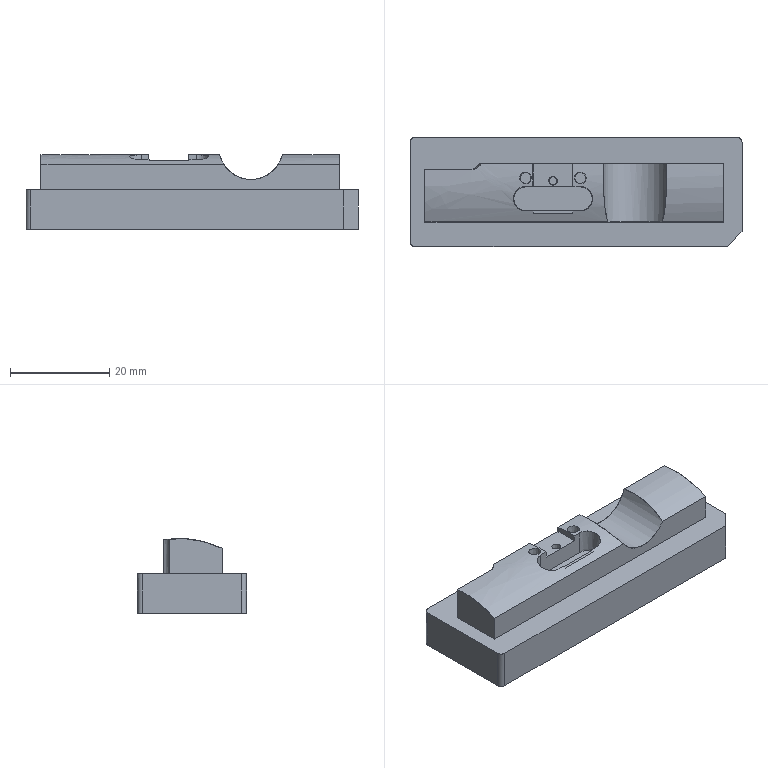NC program | PowerMill | posted with a generic post | part box 67 x 22 x 15.086 mm
Lines 3683 to 4683 of 148586:
N3780 M6
N3781 S18000 M03
N3782 G00 G90 X0.0 Y0.0
N3783 G43 Z9.7955 H15
N3784
N3785 G05 P10000 R4
N3786 X-0.8696 Y7.2678
N3787 Z0.7184
N3788 G01 Z-0.4816 F3000.0
N3789 X-0.8635 Y7.0754 F5000.0
N3790 X-0.8443 Y6.4662
N3791 X-0.4221 Y6.4795
N3792 X5.4877 Y6.4791
N3793 X5.9099 Y6.4424
N3794 X6.332 Y6.2619
N3795 X6.699 Y5.9099
N3796 X6.7541 Y5.8301
N3797 X6.9017 Y5.4877
N3798 X6.9594 Y5.0656
N3799 X6.9493 Y0.0
N3800 X6.8266 Y-0.4221
N3801 X6.7541 Y-0.5606
N3802 X6.5112 Y-0.8443
N3803 X6.332 Y-0.9949
N3804 X5.9099 Y-1.1709
N3805 X5.4877 Y-1.2145
N3806 X2.9549 Y-1.2306
N3807 X2.5328 Y-1.2027
N3808 X2.1107 Y-1.0409
N3809 X1.845 Y-0.8443
N3810 X1.5425 Y-0.5315
N3811 X1.2664 Y-0.3711
N3812 X0.8443 Y-0.2921
N3813 X0.8317 Y-0.2919
N3814 X0.8315
N3815 X-0.8443 Y-0.2674
N3816 X-1.2664 Y-0.1398
N3817 X-1.4842 Y0.0
N3818 X-1.6885 Y0.1971
N3819 X-1.8424 Y0.4221
N3820 X-1.9943 Y0.8443
N3821 X-2.0149 Y1.2664
N3822 X-2.0147 Y2.9871
N3823 X-4.0313 Y2.9866
N3824 G02 X-4.4729 Y2.5458 I-0.4407 J-0.0001
N3825 G01 X-4.8546 Y2.5466
N3826 G02 X-5.2944 Y2.988 I0.0009 J0.4407
N3827 G01 X-5.2942 Y3.1438
N3828 G02 X-4.8538 Y3.5838 I0.4407 J-0.0007
N3829 G01 X-4.4724 Y3.5841
N3830 G02 X-4.0314 Y3.1435 I0.0003 J-0.4407
N3831 G01 X-4.0313 Y2.9866
N3832 X-2.0147 Y2.9871
N3833 X-2.0145 Y5.0656
N3834 X-1.9606 Y5.4877
N3835 X-1.6885 Y5.9979
N3836 X-1.259 Y6.332
N3837 X-0.8443 Y6.4662
N3838 X-0.8635 Y7.0754
N3839 G00 Z3.8484
N3840 G01 X-13.9303 Y7.2926 F10000.0
N3841 G00 Z0.7184
N3842 G01 Z-0.4816 F3000.0
N3843 Y7.1001 F5000.0
N3844 X-13.9304 Y6.48
N3845 X-8.8648 Y6.4793
N3846 X-8.4427 Y6.46
N3847 X-8.0644 Y6.332
N3848 X-7.5984 Y5.9509
N3849 X-7.3648 Y5.4877
N3850 X-7.3108 Y5.0656
N3851 X-7.3106 Y1.2664
N3852 X-7.3319 Y0.8443
N3853 X-7.4812 Y0.4221
N3854 X-7.5984 Y0.2412
N3855 X-7.8433 Y0.0
N3856 X-8.0205 Y-0.1176
N3857 X-8.4427 Y-0.2668
N3858 X-10.1312 Y-0.2895
N3859 X-10.1441 Y-0.2919
N3860 X-10.5533 Y-0.3695
N3861 X-10.8312 Y-0.5295
N3862 X-11.1356 Y-0.8443
N3863 X-11.3976 Y-1.04
N3864 X-11.8197 Y-1.2005
N3865 X-12.2419 Y-1.23
N3866 X-18.5739 Y-1.1939
N3867 X-22.3731 Y-1.132
N3868 X-29.7609 Y-1.1249
N3869 X-30.3936 Y-1.2076
N3870 X-30.8157 Y-1.1609
N3871 X-31.2379 Y-0.9742
N3872 X-31.4044 Y-0.8443
N3873 X-31.66 Y-0.5304
N3874 X-31.7151 Y-0.4221
N3875 X-31.8364 Y0.0
N3876 X-31.8467 Y0.4221
N3877 Y4.2213
N3878 X-31.8399 Y4.6435
N3879 X-31.7279 Y5.0656
N3880 X-31.66 Y5.198
N3881 X-31.4339 Y5.4877
N3882 X-31.2379 Y5.6466
N3883 X-30.8157 Y5.8349
N3884 X-30.3936 Y5.8775
N3885 X-21.1067
N3886 X-21.0966 Y5.8789
N3887 X-20.8747 Y5.9099
N3888 X-20.6845 Y5.9891
N3889 X-20.2624 Y6.3017
N3890 X-19.8403 Y6.4525
N3891 X-18.996 Y6.4808
N3892 X-13.9304 Y6.48
N3893 X-13.9303 Y7.1001
N3894 G00 Z3.7118
N3895 G01 X-1.7244 Y-0.8629 F10000.0
N3896 G00 Z0.5818
N3897 G01 Z-0.6182 F3000.0
N3898 X-1.6213 Y-0.7004 F5000.0
N3899 X-1.2664 Y-0.1409
N3900 X-1.4885 Y0.0
N3901 X-1.6885 Y0.1953
N3902 X-1.8436 Y0.4221
N3903 X-1.9943 Y0.8443
N3904 X-2.0149 Y1.2664
N3905 X-2.0145 Y5.0656
N3906 X-2.0144 Y5.4879
N3907 X-1.9993 Y5.9099
N3908 X-1.8637 Y6.332
N3909 X-1.6885 Y6.5944
N3910 X-1.5284 Y6.7541
N3911 X-1.2664 Y6.9281
N3912 X-0.8443 Y7.0629
N3913 X-0.4221 Y7.0775
N3914 X5.4877
N3915 X5.9099 Y7.0484
N3916 X6.332 Y6.8846
N3917 X6.5162 Y6.7541
N3918 X6.7541 Y6.4929
N3919 X6.8515 Y6.332
N3920 X6.9871 Y5.9099
N3921 X7.001 Y5.4877
N3922 X7.0095 Y0.4221
N3923 X6.9942 Y-0.8443
N3924 X6.9033 Y-1.2664
N3925 X6.7541 Y-1.5538
N3926 X6.6422 Y-1.6885
N3927 X6.332 Y-1.9496
N3928 X5.9378 Y-2.1107
N3929 X5.4877 Y-2.1433
N3930 X3.3771 Y-2.1495
N3931 X2.9549 Y-2.1158
N3932 X2.5328 Y-1.9343
N3933 X2.231 Y-1.6885
N3934 X2.1107 Y-1.5345
N3935 X1.9706 Y-1.2664
N3936 X1.8103 Y-0.8443
N3937 X1.7156 Y-0.7104
N3938 X1.5636 Y-0.5532
N3939 X1.5416 Y-0.5322
N3940 X1.2664 Y-0.3723
N3941 X0.8443 Y-0.2944
N3942 X0.8319 Y-0.2943
N3943 X-0.8443 Y-0.2707
N3944 X-1.2664 Y-0.1409
N3945 X-1.6213 Y-0.7004
N3946 G00 Z3.7118
N3947 G01 X-32.4909 Y5.4568 F10000.0
N3948 G00 Z0.5818
N3949 G01 Z-0.6182 F3000.0
N3950 X-32.3196 Y5.369 F5000.0
N3951 X-31.7279 Y5.0656
N3952 X-31.66 Y5.198
N3953 X-31.4339 Y5.4877
N3954 X-31.2379 Y5.6466
N3955 X-30.8157 Y5.8349
N3956 X-30.3936 Y5.8775
N3957 X-21.1067 Y5.88
N3958 X-20.8748 Y5.9099
N3959 X-20.6845 Y5.9907
N3960 X-20.5063 Y6.1375
N3961 X-20.2624 Y6.509
N3962 X-20.0356 Y6.7541
N3963 X-19.8403 Y6.8912
N3964 X-19.4181 Y7.0463
N3965 X-18.996 Y7.0775
N3966 X-8.8648
N3967 X-8.4427 Y7.0562
N3968 X-8.0205 Y6.9075
N3969 X-7.7965 Y6.7541
N3970 X-7.5984 Y6.5481
N3971 X-7.4621 Y6.332
N3972 X-7.3251 Y5.9099
N3973 X-7.3103 Y5.4877
N3974 X-7.3102 Y3.5191
N3975 X-5.3455 Y3.522
N3976 G02 X-4.7413 Y4.1229 I0.6 J0.0009
N3977 G01 X-4.576 Y4.1217
N3978 G02 X-3.9802 Y3.5223 I-0.0042 J-0.6
N3979 G01 X-3.9799 Y3.2599
N3980 G02 X-4.5789 Y2.6593 I-0.6 J-0.0006
N3981 G01 X-4.7441 Y2.6591
N3982 G02 X-5.3451 Y3.2582 I-0.001 J0.6
N3983 G01 X-5.3455 Y3.522
N3984 X-7.3102 Y3.5191
N3985 X-7.3101 Y1.2664
N3986 X-7.3308 Y0.8443
N3987 X-7.4792 Y0.4221
N3988 X-7.5984 Y0.2388
N3989 X-7.8393 Y0.0
N3990 X-8.0205 Y-0.1202
N3991 X-8.4427 Y-0.2691
N3992 X-10.1312 Y-0.294
N3993 X-10.5533 Y-0.3709
N3994 X-10.8301 Y-0.5302
N3995 X-10.85 Y-0.549
N3996 X-11.0063 Y-0.7105
N3997 X-11.0127 Y-0.7196
N3998 X-11.1013 Y-0.8443
N3999 X-11.2616 Y-1.2664
N4000 X-11.3976 Y-1.5291
N4001 X-11.5249 Y-1.6885
N4002 X-11.8197 Y-1.9378
N4003 X-12.2952 Y-2.1107
N4004 X-12.664 Y-2.1461
N4005 X-18.1517 Y-2.121
N4006 X-30.3936 Y-2.1116
N4007 X-30.8157 Y-2.0767
N4008 X-31.2379 Y-1.886
N4009 X-31.4652 Y-1.6885
N4010 X-31.66 Y-1.4388
N4011 X-31.7414 Y-1.2664
N4012 X-31.8427 Y-0.8443
N4013 X-31.8467 Y-0.4221
N4014 Y4.2213
N4015 X-31.8399 Y4.6435
N4016 X-31.7279 Y5.0656
N4017 X-32.3196 Y5.369
N4018 G00 Z3.5751
N4019 G01 X-1.7255 Y-0.8634 F10000.0
N4020 G00 Z0.4451
N4021 G01 Z-0.7549 F3000.0
N4022 X-1.6221 Y-0.7009 F5000.0
N4023 X-1.2664 Y-0.1419
N4024 X-1.4895 Y0.0
N4025 X-1.6885 Y0.1935
N4026 X-1.8448 Y0.4221
N4027 X-1.9944 Y0.8443
N4028 X-2.0149 Y1.2664
N4029 X-2.0147 Y3.2969
N4030 X-3.98 Y3.2671
N4031 G02 X-4.5789 Y2.658 I-0.6 J-0.0091
N4032 G01 X-4.7435 Y2.6577
N4033 G02 X-5.3444 Y3.2732 I-0.0011 J0.6
N4034 G01 X-5.3371 Y3.5541
N4035 G02 X-4.7074 Y4.1379 I0.5998 J-0.0154
N4036 G01 X-4.5542 Y4.1303
N4037 G02 X-3.9842 Y3.5401 I-0.0299 J-0.5993
N4038 G01 X-3.98 Y3.2671
N4039 X-2.0147 Y3.2969
N4040 X-2.0144 Y5.4877
N4041 X-1.9993 Y5.9099
N4042 X-1.8637 Y6.332
N4043 X-1.6885 Y6.5944
N4044 X-1.5284 Y6.7541
N4045 X-1.2664 Y6.9281
N4046 X-0.8443 Y7.0629
N4047 X-0.4221 Y7.0775
N4048 X5.4877
N4049 X5.9099 Y7.057
N4050 X6.332 Y6.9103
N4051 X6.5628 Y6.7541
N4052 X6.7541 Y6.5556
N4053 X6.8982 Y6.332
N4054 X7.0338 Y5.9099
N4055 X7.0455 Y5.4877
N4056 X7.0499 Y-0.8443
N4057 X7.0217 Y-1.6885
N4058 X6.8839 Y-2.1107
N4059 X6.7541 Y-2.3121
N4060 X6.542 Y-2.5328
N4061 X6.332 Y-2.6769
N4062 X5.9099 Y-2.8265
N4063 X5.4877 Y-2.8518
N4064 X3.3771 Y-2.851
N4065 X2.9549 Y-2.799
N4066 X2.5328 Y-2.5985
N4067 X2.453 Y-2.5328
N4068 X2.1086 Y-2.1107
N4069 X1.9675 Y-1.6885
N4070 X1.9449 Y-1.2664
N4071 X1.9425 Y-1.2551
N4072 X1.9117 Y-1.1111
N4073 X1.8196 Y-0.8686
N4074 X1.8089 Y-0.8443
N4075 X1.7105 Y-0.705
N4076 X1.5856 Y-0.5758
N4077 X1.5405 Y-0.5329
N4078 X1.2664 Y-0.3736
N4079 X0.8443 Y-0.2956
N4080 X-0.8443 Y-0.2739
N4081 X-1.2664 Y-0.1419
N4082 X-1.6221 Y-0.7009
N4083 G00 Z3.5751
N4084 G01 X-32.4909 Y5.4568 F10000.0
N4085 G00 Z0.4451
N4086 G01 Z-0.7549 F3000.0
N4087 X-32.3196 Y5.369 F5000.0
N4088 X-31.7279 Y5.0656
N4089 X-31.66 Y5.198
N4090 X-31.4339 Y5.4877
N4091 X-31.2379 Y5.6466
N4092 X-30.8157 Y5.8349
N4093 X-30.3936 Y5.8775
N4094 X-21.1067 Y5.8809
N4095 X-20.8815 Y5.9099
N4096 X-20.6845 Y5.9953
N4097 X-20.5103 Y6.1406
N4098 X-20.2624 Y6.5185
N4099 X-20.0428 Y6.7541
N4100 X-19.8403 Y6.8955
N4101 X-19.4181 Y7.051
N4102 X-18.996 Y7.0775
N4103 X-8.8648
N4104 X-8.4427 Y7.0564
N4105 X-8.0205 Y6.9085
N4106 X-7.7959 Y6.7541
N4107 X-7.5984 Y6.5488
N4108 X-7.4609 Y6.332
N4109 X-7.3245 Y5.9099
N4110 X-7.3097 Y5.4877
N4111 X-7.3095 Y1.2664
N4112 X-7.3297 Y0.8443
N4113 X-7.4772 Y0.4221
N4114 X-7.5984 Y0.2363
N4115 X-7.8353 Y0.0
N4116 X-8.0205 Y-0.1229
N4117 X-8.4427 Y-0.2713
N4118 X-10.1312 Y-0.2952
N4119 X-10.5533 Y-0.3723
N4120 X-10.8291 Y-0.5309
N4121 X-10.8696 Y-0.5691
N4122 X-11.001 Y-0.705
N4123 X-11.0075 Y-0.7141
N4124 X-11.0999 Y-0.8443
N4125 X-11.1106 Y-0.8686
N4126 X-11.2035 Y-1.1133
N4127 X-11.2371 Y-1.2664
N4128 X-11.2576 Y-1.6885
N4129 X-11.3976 Y-2.1212
N4130 X-11.7436 Y-2.5328
N4131 X-11.8197 Y-2.5957
N4132 X-12.2419 Y-2.8008
N4133 X-12.664 Y-2.8513
N4134 X-30.3936 Y-2.8507
N4135 X-30.8157 Y-2.8049
N4136 X-31.2379 Y-2.6198
N4137 X-31.3527 Y-2.5328
N4138 X-31.66 Y-2.1712
N4139 X-31.8307 Y-1.6885
N4140 X-31.8467 Y-1.2664
N4141 Y4.2213
N4142 X-31.8399 Y4.6435
N4143 X-31.7279 Y5.0656
N4144 X-32.3196 Y5.369
N4145 G00 Z3.4385
N4146 G01 X-1.7265 Y-0.8637 F10000.0
N4147 G00 Z0.3085
N4148 G01 Z-0.8915 F3000.0
N4149 X-1.6229 Y-0.7015 F5000.0
N4150 X-1.2664 Y-0.143
N4151 X-1.4904 Y0.0
N4152 X-1.6885 Y0.1917
N4153 X-1.846 Y0.4221
N4154 X-1.9944 Y0.8443
N4155 X-2.0149 Y1.2664
N4156 X-2.0147 Y3.2807
N4157 X-3.98 Y3.2624
N4158 G02 X-4.5789 Y2.6568 I-0.6 J-0.0056
N4159 G01 X-4.7429 Y2.6565
N4160 G02 X-5.3438 Y3.2719 I-0.0011 J0.6
N4161 G01 X-5.3365 Y3.554
N4162 G02 X-4.712 Y4.1381 I0.5998 J-0.0154
N4163 G01 X-4.5578 Y4.1317
N4164 G02 X-3.9826 Y3.5378 I-0.0248 J-0.5995
N4165 G01 X-3.98 Y3.2624
N4166 X-2.0147 Y3.2807
N4167 X-2.0144 Y5.4877
N4168 X-1.9993 Y5.9099
N4169 X-1.8637 Y6.332
N4170 X-1.6885 Y6.5944
N4171 X-1.5284 Y6.7541
N4172 X-1.2664 Y6.9281
N4173 X-0.8443 Y7.0629
N4174 X-0.4221 Y7.0775
N4175 X5.4877
N4176 X5.9099 Y7.0647
N4177 X6.332 Y6.9358
N4178 X6.6094 Y6.7541
N4179 X6.7541 Y6.6115
N4180 X6.9449 Y6.332
N4181 X7.0805 Y5.9099
N4182 X7.09 Y5.4877
N4183 X7.0928 Y-0.4221
N4184 X7.0807 Y-2.1107
N4185 X7.0012 Y-2.5328
N4186 X6.7541 Y-2.9638
N4187 X6.332 Y-3.2951
N4188 X6.1339 Y-3.3771
N4189 X5.9099 Y-3.4316
N4190 X3.3771 Y-3.4431
N4191 X2.9549 Y-3.4169
N4192 X2.7996 Y-3.3771
N4193 X2.5328 Y-3.2572
N4194 X2.1724 Y-2.9549
N4195 X2.1107 Y-2.8782
N4196 X1.9299 Y-2.5328
N4197 X1.8478 Y-2.1107
N4198 X1.9424 Y-1.4792
N4199 X1.9433 Y-1.2664
N4200 X1.9086 Y-1.1028
N4201 X1.8287 Y-0.8924
N4202 X1.8272 Y-0.889
N4203 X1.8076 Y-0.8443
N4204 X1.7053 Y-0.6996
N4205 X1.6082 Y-0.5992
N4206 X1.5395 Y-0.5336
N4207 X1.2664 Y-0.3748
N4208 X0.8443 Y-0.2968
N4209 X-0.8443 Y-0.2772
N4210 X-1.2664 Y-0.143
N4211 X-1.6229 Y-0.7015
N4212 G00 Z3.4385
N4213 G01 X-32.4909 Y5.4568 F10000.0
N4214 G00 Z0.3085
N4215 G01 Z-0.8915 F3000.0
N4216 X-32.3196 Y5.369 F5000.0
N4217 X-31.7279 Y5.0656
N4218 X-31.66 Y5.198
N4219 X-31.4339 Y5.4877
N4220 X-31.2379 Y5.6467
N4221 X-30.8157 Y5.8349
N4222 X-30.3936 Y5.8775
N4223 X-30.2495
N4224 X-21.2958 Y5.8807
N4225 X-21.1067 Y5.8817
N4226 X-20.8887 Y5.9099
N4227 X-20.6845 Y5.9998
N4228 X-20.5144 Y6.1437
N4229 X-20.2624 Y6.528
N4230 X-20.0499 Y6.7541
N4231 X-19.8403 Y6.8999
N4232 X-19.4181 Y7.0541
N4233 X-18.996 Y7.0775
N4234 X-8.8648
N4235 X-8.4427 Y7.0566
N4236 X-8.0205 Y6.9089
N4237 X-7.7953 Y6.7541
N4238 X-7.5984 Y6.5496
N4239 X-7.4598 Y6.332
N4240 X-7.324 Y5.9099
N4241 X-7.3091 Y5.4877
N4242 X-7.309 Y1.2664
N4243 X-7.3288 Y0.8443
N4244 X-7.4753 Y0.4221
N4245 X-7.5984 Y0.2342
N4246 X-7.8315 Y0.0
N4247 X-8.0205 Y-0.1255
N4248 X-8.4427 Y-0.2731
N4249 X-10.1312 Y-0.2964
N4250 X-10.5533 Y-0.3736
N4251 X-10.8281 Y-0.5316
N4252 X-10.9756 Y-0.6773
N4253 X-11.0986 Y-0.8443
N4254 X-11.1197 Y-0.8925
N4255 X-11.1989 Y-1.1012
N4256 X-11.2332 Y-1.2664
N4257 X-11.2334 Y-1.4794
N4258 X-11.1383 Y-2.1107
N4259 X-11.2192 Y-2.5328
N4260 X-11.3976 Y-2.8762
N4261 X-11.4609 Y-2.9549
N4262 X-11.8197 Y-3.2536
N4263 X-12.0819 Y-3.3771
N4264 X-12.2419 Y-3.4147
N4265 X-12.664 Y-3.4457
N4266 X-29.9715 Y-3.4146
N4267 X-30.3936 Y-3.4319
N4268 X-30.8157 Y-3.3916
N4269 X-31.2379 Y-3.201
N4270 X-31.514 Y-2.9549
N4271 X-31.66 Y-2.7547
N4272 X-31.7626 Y-2.5328
N4273 X-31.8454 Y-2.1107
N4274 X-31.8455 Y-1.2963
N4275 X-31.8456 Y-1.2935
N4276 X-31.8467 Y-1.2664
N4277 Y3.9809
N4278 Y4.2213
N4279 X-31.8399 Y4.6435
N4280 X-31.7279 Y5.0656
N4281 X-32.3196 Y5.369
N4282 G00 Z3.3019
N4283 G01 X-1.7275 Y-0.8641 F10000.0
N4284 G00 Z0.1719
N4285 G01 Z-1.0281 F3000.0
N4286 X-1.6237 Y-0.702 F5000.0
N4287 X-1.2664 Y-0.1441
N4288 X-1.4914 Y0.0
N4289 X-1.6885 Y0.1901
N4290 X-1.8467 Y0.4221
N4291 X-1.9944 Y0.8443
N4292 X-2.0149 Y1.2664
N4293 X-2.0147 Y3.2948
N4294 X-3.9801 Y3.2647
N4295 G02 X-4.5789 Y2.6555 I-0.5999 J-0.0092
N4296 G01 X-4.7423 Y2.6552
N4297 G02 X-5.3433 Y3.2704 I-0.0011 J0.6
N4298 G01 X-5.3361 Y3.5534
N4299 G02 X-4.7083 Y4.1376 I0.5998 J-0.0151
N4300 G01 X-4.5562 Y4.1305
N4301 G02 X-3.9843 Y3.5403 I-0.028 J-0.5993
N4302 G01 X-3.9801 Y3.2647
N4303 X-2.0147 Y3.2948
N4304 X-2.0145 Y5.4877
N4305 X-1.9994 Y5.9099
N4306 X-1.8637 Y6.332
N4307 X-1.6885 Y6.5944
N4308 X-1.5284 Y6.7541
N4309 X-1.2664 Y6.9281
N4310 X-0.8443 Y7.0629
N4311 X-0.4221 Y7.0775
N4312 X5.4877
N4313 X5.9099 Y7.0694
N4314 X6.332 Y6.9571
N4315 X6.6561 Y6.7541
N4316 X6.7541 Y6.6618
N4317 X6.9916 Y6.332
N4318 X7.1271 Y5.9099
N4319 X7.1345 Y5.4877
N4320 X7.1367 Y-1.6885
N4321 X7.1324 Y-2.5328
N4322 X7.0794 Y-2.9549
N4323 X6.8817 Y-3.3771
N4324 X6.7541 Y-3.5383
N4325 X6.4159 Y-3.7992
N4326 X6.332 Y-3.8418
N4327 X5.9099 Y-3.9594
N4328 X2.9549 Y-3.9643
N4329 X2.5328 Y-3.8847
N4330 X2.344 Y-3.7992
N4331 X2.1107 Y-3.6378
N4332 X1.872 Y-3.3771
N4333 X1.6885 Y-3.0003
N4334 X1.6285 Y-2.5328
N4335 X1.6885 Y-2.1932
N4336 X1.899 Y-1.6885
N4337 X1.9412 Y-1.4793
N4338 X1.9418 Y-1.2664
N4339 X1.9055 Y-1.0946
N4340 X1.8376 Y-0.9158
N4341 X1.8361 Y-0.9124
N4342 X1.8063 Y-0.8443
N4343 X1.7002 Y-0.6943
N4344 X1.6317 Y-0.6234
N4345 X1.5384 Y-0.5343
N4346 X1.2664 Y-0.3761
N4347 X0.8443 Y-0.298
N4348 X-0.8443 Y-0.2804
N4349 X-1.2664 Y-0.1441
N4350 X-1.6237 Y-0.702
N4351 G00 Z3.3019
N4352 G01 X-32.4909 Y5.4568 F10000.0
N4353 G00 Z0.1719
N4354 G01 Z-1.0281 F3000.0
N4355 X-32.3196 Y5.369 F5000.0
N4356 X-31.7279 Y5.0656
N4357 X-31.66 Y5.198
N4358 X-31.4339 Y5.4877
N4359 X-31.2379 Y5.6467
N4360 X-30.8157 Y5.8349
N4361 X-30.3936 Y5.8775
N4362 X-30.1067
N4363 X-21.2958 Y5.8807
N4364 X-21.095 Y5.884
N4365 X-20.8959 Y5.9099
N4366 X-20.6845 Y6.0044
N4367 X-20.5185 Y6.1469
N4368 X-20.2624 Y6.5375
N4369 X-20.0571 Y6.7541
N4370 X-19.8403 Y6.904
N4371 X-19.4181 Y7.0554
N4372 X-18.996 Y7.0775
N4373 X-8.8648
N4374 X-8.4427 Y7.0568
N4375 X-8.0205 Y6.9092
N4376 X-7.7946 Y6.7541
N4377 X-7.5984 Y6.5503
N4378 X-7.459 Y6.332
N4379 X-7.3235 Y5.9099
N4380 X-7.3086 Y5.4877
N4381 X-7.3085 Y1.2664
N4382 X-7.3281 Y0.8443
N4383 X-7.4741 Y0.4221
N4384 X-7.5984 Y0.2324
N4385 X-7.8294 Y0.0
N4386 X-8.0205 Y-0.1281
N4387 X-8.4427 Y-0.2744
N4388 X-10.1312 Y-0.2976
N4389 X-10.5533 Y-0.3748
N4390 X-10.827 Y-0.5323
N4391 X-10.9746 Y-0.6774
N4392 X-11.0973 Y-0.8443
N4393 X-11.1287 Y-0.9159
N4394 X-11.1962 Y-1.0937
N4395 X-11.232 Y-1.2664
N4396 X-11.2322 Y-1.4795
N4397 X-11.19 Y-1.6885
N4398 X-11.0095 Y-2.1107
N4399 X-10.9213 Y-2.5328
N4400 X-10.9677 Y-2.9549
N4401 X-11.1655 Y-3.3771
N4402 X-11.3976 Y-3.6377
N4403 X-11.6415 Y-3.7992
N4404 X-11.8197 Y-3.8841
N4405 X-12.2419 Y-3.9636
N4406 X-21.1081 Y-3.9339
N4407 X-29.9744 Y-3.9186
N4408 X-30.3936 Y-3.9347
N4409 X-30.8157 Y-3.8946
N4410 X-31.0748 Y-3.7992
N4411 X-31.2379 Y-3.7042
N4412 X-31.5817 Y-3.3771
N4413 X-31.66 Y-3.2577
N4414 X-31.7904 Y-2.9549
N4415 X-31.8467 Y-2.5328
N4416 Y4.2213
N4417 X-31.8399 Y4.6435
N4418 X-31.7279 Y5.0656
N4419 X-32.3196 Y5.369
N4420 G00 Z3.1653
N4421 G01 X-1.7317 Y-0.8694 F10000.0
N4422 G00 Z0.0353
N4423 G01 Z-1.1647 F3000.0
N4424 X-1.6276 Y-0.7075 F5000.0
N4425 X-1.2664 Y-0.1452
N4426 X-1.4924 Y0.0
N4427 X-1.6885 Y0.1885
N4428 X-1.8468 Y0.4221
N4429 X-1.9944 Y0.8443
N4430 X-2.0149 Y1.2664
N4431 X-2.0145 Y5.4877
N4432 X-1.9994 Y5.9099
N4433 X-1.8637 Y6.332
N4434 X-1.6885 Y6.5944
N4435 X-1.5284 Y6.7541
N4436 X-1.2664 Y6.9282
N4437 X-0.8443 Y7.0629
N4438 X-0.4221 Y7.0775
N4439 X-0.3265
N4440 X5.4877
N4441 X5.6563 Y7.0742
N4442 X5.9099 Y7.0741
N4443 X6.332 Y6.9778
N4444 X6.7027 Y6.7541
N4445 X7.0382 Y6.332
N4446 X7.1738 Y5.9099
N4447 X7.1796 Y5.4877
N4448 X7.1805 Y-2.9549
N4449 X7.1421 Y-3.3771
N4450 X6.9634 Y-3.7992
N4451 X6.7541 Y-4.0573
N4452 X6.5384 Y-4.2213
N4453 X6.332 Y-4.3322
N4454 X5.9099 Y-4.4291
N4455 X2.5328 Y-4.432
N4456 X2.1107 Y-4.329
N4457 X1.9094 Y-4.2213
N4458 X1.6885 Y-4.0522
N4459 X1.4852 Y-3.7992
N4460 X1.3086 Y-3.3771
N4461 X1.2778 Y-2.9549
N4462 X1.3819 Y-2.5328
N4463 X1.8028 Y-1.9194
N4464 X1.884 Y-1.7245
N4465 X1.8977 Y-1.6885
N4466 X1.94 Y-1.4793
N4467 X1.9402 Y-1.2664
N4468 X1.9025 Y-1.0866
N4469 X1.8464 Y-0.9387
N4470 X1.8049 Y-0.8443
N4471 X1.6951 Y-0.6889
N4472 X1.656 Y-0.6484
N4473 X1.5374 Y-0.5349
N4474 X1.2664 Y-0.3773
N4475 X0.8443 Y-0.2992
N4476 X0.8315 Y-0.2991
N4477 X-0.8443 Y-0.2836
N4478 X-1.2664 Y-0.1452
N4479 X-1.6276 Y-0.7075
N4480 G00 Z3.1653
N4481 G01 X-32.4909 Y5.4568 F10000.0
N4482 G00 Z0.0353
N4483 G01 Z-1.1647 F3000.0
N4484 X-32.3196 Y5.369 F5000.0
N4485 X-31.7279 Y5.0656
N4486 X-31.66 Y5.198
N4487 X-31.4339 Y5.4877
N4488 X-31.2379 Y5.6467
N4489 X-30.8157 Y5.8349
N4490 X-30.3936 Y5.8775
N4491 X-29.9626
N4492 X-21.3009 Y5.8806
N4493 X-21.1067 Y5.8833
N4494 X-20.903 Y5.9099
N4495 X-20.6845 Y6.009
N4496 X-20.5226 Y6.15
N4497 X-20.2624 Y6.547
N4498 X-20.0643 Y6.7541
N4499 X-19.8403 Y6.9077
N4500 X-19.4181 Y7.0567
N4501 X-18.996 Y7.0775
N4502 X-8.8648
N4503 X-8.4427 Y7.057
N4504 X-8.0205 Y6.9095
N4505 X-7.794 Y6.7541
N4506 X-7.5984 Y6.5511
N4507 X-7.4585 Y6.332
N4508 X-7.3229 Y5.9099
N4509 X-7.308 Y5.4877
N4510 Y3.5203
N4511 X-5.3431 Y3.5222
N4512 G02 X-4.7398 Y4.1227 I0.6 J0.0005
N4513 G01 X-4.5769 Y4.1218
N4514 G02 X-3.9802 Y3.5222 I-0.0033 J-0.6
N4515 G01 X-3.98 Y3.2546
N4516 G02 X-4.5788 Y2.6543 I-0.6 J-0.0003
N4517 G01 X-4.7417 Y2.654
N4518 G02 X-5.3429 Y3.2534 I-0.0012 J0.6
N4519 G01 X-5.3431 Y3.5222
N4520 X-7.308 Y3.5203
N4521 X-7.3079 Y1.2664
N4522 X-7.3273 Y0.8443
N4523 X-7.473 Y0.4221
N4524 X-7.5984 Y0.2305
N4525 X-7.8274 Y0.0
N4526 X-8.0205 Y-0.1307
N4527 X-8.4427 Y-0.2756
N4528 X-10.1312 Y-0.2988
N4529 X-10.5533 Y-0.3761
N4530 X-10.826 Y-0.533
N4531 X-10.9321 Y-0.6335
N4532 X-10.9855 Y-0.6887
N4533 X-11.0959 Y-0.8443
N4534 X-11.1808 Y-1.0498
N4535 X-11.2308 Y-1.2664
N4536 X-11.231 Y-1.4795
N4537 X-11.1887 Y-1.6885
N4538 X-11.1705 Y-1.7342
N4539 X-11.0848 Y-1.9346
N4540 X-11.0765 Y-1.9468
N4541 X-10.6722 Y-2.5328
N4542 X-10.569 Y-2.9549
N4543 X-10.598 Y-3.3771
N4544 X-10.7731 Y-3.7992
N4545 X-10.9755 Y-4.0434
N4546 X-11.1959 Y-4.2213
N4547 X-11.3976 Y-4.3258
N4548 X-11.8197 Y-4.432
N4549 X-30.3936 Y-4.4232
N4550 X-30.8157 Y-4.3791
N4551 X-31.1845 Y-4.2213
N4552 X-31.6241 Y-3.7992
N4553 X-31.8058 Y-3.3771
N4554 X-31.8467 Y-2.9549
N4555 Y4.2213
N4556 X-31.8399 Y4.6435
N4557 X-31.7279 Y5.0656
N4558 X-32.3196 Y5.369
N4559 G00 Z3.0286
N4560 G01 X-2.2961 Y7.2035 F10000.0
N4561 G00 Z-0.1014
N4562 G01 Z-1.3014 F3000.0
N4563 X-2.1601 Y7.0672 F5000.0
N4564 X-1.6885 Y6.5945
N4565 X-1.5285 Y6.7541
N4566 X-1.2664 Y6.9282
N4567 X-0.8443 Y7.0629
N4568 X-0.4221 Y7.0775
N4569 X0.6036 Y7.0774
N4570 X5.4877
N4571 X5.5135 Y7.0769
N4572 X5.9099
N4573 X6.332 Y6.9972
N4574 X6.7541 Y6.753
N4575 X7.0889 Y6.332
N4576 X7.1763 Y6.1175
N4577 X7.2245 Y5.9099
N4578 X7.2401 Y4.2213
N4579 X7.2416 Y-3.3771
N4580 X7.1978 Y-3.7992
N4581 X7.0229 Y-4.2213
N4582 X6.7541 Y-4.5357
N4583 X6.6094 Y-4.6435
N4584 X6.332 Y-4.7826
N4585 X5.9099 Y-4.8646
N4586 X2.1107 Y-4.8679
N4587 X1.6885 Y-4.8142
N4588 X1.3262 Y-4.6435
N4589 X0.9118 Y-4.2213
N4590 X0.8443 Y-4.0991
N4591 X0.7363 Y-3.7992
N4592 X0.7112 Y-3.3771
N4593 X0.8169 Y-2.9549
N4594 X1.1036 Y-2.5328
N4595 X1.6572 Y-2.1107
N4596 X1.7369 Y-2.0155
N4597 X1.7658 Y-1.9734
N4598 X1.8965 Y-1.6885
N4599 X1.9388 Y-1.4793
N4600 X1.9386 Y-1.2664
N4601 X1.8996 Y-1.0787
N4602 X1.8546 Y-0.9603
N4603 X1.8036 Y-0.8443
N4604 X1.6967 Y-0.693
N4605 X1.688 Y-0.6819
N4606 X1.6783 Y-0.6717
N4607 X1.5363 Y-0.5356
N4608 X1.2664 Y-0.3785
N4609 X0.8443 Y-0.3004
N4610 X-0.8443 Y-0.2868
N4611 X-1.2664 Y-0.1463
N4612 X-1.4934 Y0.0
N4613 X-1.6885 Y0.1869
N4614 X-1.847 Y0.4221
N4615 X-1.9944 Y0.8443
N4616 X-2.0149 Y1.2664
N4617 X-2.0145 Y5.4877
N4618 X-1.9994 Y5.9099
N4619 X-1.8638 Y6.332
N4620 X-1.6885 Y6.5945
N4621 X-2.1601 Y7.0672
N4622 G00 Z3.0286
N4623 G01 X-32.4909 Y5.4568 F10000.0
N4624 G00 Z-0.1014
N4625 G01 Z-1.3014 F3000.0
N4626 X-32.3196 Y5.369 F5000.0
N4627 X-31.7279 Y5.0656
N4628 X-31.66 Y5.198
N4629 X-31.4339 Y5.4877
N4630 X-31.2379 Y5.6467
N4631 X-30.8157 Y5.8349
N4632 X-30.3936 Y5.8775
N4633 X-29.8184
N4634 X-21.333 Y5.8806
N4635 X-21.1067 Y5.8841
N4636 X-20.9102 Y5.9099
N4637 X-20.6845 Y6.0135
N4638 X-20.5267 Y6.1531
N4639 X-20.2624 Y6.5565
N4640 X-20.0715 Y6.7541
N4641 X-19.8403 Y6.9114
N4642 X-19.4181 Y7.058
N4643 X-18.996 Y7.0775
N4644 X-8.8648
N4645 X-8.4427 Y7.0572
N4646 X-8.0205 Y6.9098
N4647 X-7.7933 Y6.7541
N4648 X-7.5984 Y6.5522
N4649 X-7.458 Y6.332
N4650 X-7.3224 Y5.9099
N4651 X-7.3074 Y5.4877
N4652 Y3.5221
N4653 X-5.3426 Y3.5228
N4654 G02 X-4.7393 Y4.123 I0.6 J0.0002
N4655 G01 X-4.5769 Y4.1221
N4656 G02 X-3.9802 Y3.5227 I-0.0033 J-0.6
N4657 G01 X-3.9799 Y3.2117
N4658 G02 X-4.5788 Y2.6112 I-0.6 J-0.0005
N4659 G01 X-4.7413 Y2.6109
N4660 G02 X-5.3425 Y3.2106 I-0.0012 J0.6
N4661 G01 X-5.3426 Y3.5228
N4662 X-7.3074 Y3.5221
N4663 Y1.2664
N4664 X-7.3266 Y0.8443
N4665 X-7.4718 Y0.4221
N4666 X-7.5984 Y0.2286
N4667 X-7.8254 Y0.0
N4668 X-8.0205 Y-0.1333
N4669 X-8.4427 Y-0.2769
N4670 X-10.1312 Y-0.3
N4671 X-10.5533 Y-0.3773
N4672 X-10.8249 Y-0.5336
N4673 X-10.9543 Y-0.6564
N4674 X-10.9803 Y-0.6833
N4675 X-11.0946 Y-0.8443
N4676 X-11.18 Y-1.0496
N4677 X-11.2296 Y-1.2664
N4678 X-11.2298 Y-1.4796
N4679 X-11.1875 Y-1.6885
N4680 X-11.1592 Y-1.7608
N4681 X-11.0936 Y-1.9142
N4682 X-10.9492 Y-2.1107
N4683 X-10.4079 Y-2.5328
N4684 X-10.1312 Y-2.9357
N4685 X-10.0129 Y-3.3771
N4686 X-10.0371 Y-3.7992
N4687 X-10.212 Y-4.2213
N4688 X-10.6309 Y-4.6435
N4689 X-10.9755 Y-4.8077
N4690 X-11.3976 Y-4.8669
N4691 X-29.9715 Y-4.8456
N4692 X-29.9736
N4693 X-30.3936 Y-4.8571
N4694 X-30.8157 Y-4.817
N4695 X-31.2121 Y-4.6435
N4696 X-31.6325 Y-4.2213
N4697 X-31.8098 Y-3.7992
N4698 X-31.8467 Y-3.3771
N4699 Y4.2213
N4700 X-31.8399 Y4.6435
N4701 X-31.7279 Y5.0656
N4702 X-32.3196 Y5.369
N4703 G00 Z2.892
N4704 G01 X-2.2961 Y7.2036 F10000.0
N4705 G00 Z-0.238
N4706 G01 Z-1.438 F3000.0
N4707 X-2.1602 Y7.0673 F5000.0
N4708 X-1.6885 Y6.5945
N4709 X-1.5285 Y6.7541
N4710 X-1.2664 Y6.9282
N4711 X-0.8443 Y7.0629
N4712 X-0.4221 Y7.0775
N4713 X5.9099
N4714 X6.332 Y7.0167
N4715 X6.8144 Y6.7541
N4716 X7.1499 Y6.332
N4717 X7.2859 Y5.9099
N4718 X7.3046 Y-3.7992
N4719 X7.2504 Y-4.2213
N4720 X7.1763 Y-4.4375
N4721 X7.0654 Y-4.6435
N4722 X6.7541 Y-4.9805
N4723 X6.6275 Y-5.0656
N4724 X6.332 Y-5.2005
N4725 X5.9099 Y-5.264
N4726 X-0.8443 Y-5.2488
N4727 X-1.2664 Y-5.1129
N4728 X-1.6885 Y-4.7767
N4729 X-1.7861 Y-4.6435
N4730 X-1.9704 Y-4.2213
N4731 X-2.0107 Y-3.7992
N4732 X-1.9375 Y-3.3771
N4733 X-1.6885 Y-2.9432
N4734 X-1.2664 Y-2.6072
N4735 X-1.1104 Y-2.5328
N4736 X-0.8443 Y-2.4738
N4737 X0.8443 Y-2.4587
N4738 X1.2664 Y-2.376
N4739 X1.4645 Y-2.2576
N4740 X1.6237 Y-2.1362
N4741 X1.742 Y-2.0046
N4742 X1.7554 Y-1.9872
N4743 X1.766 Y-1.9681
N4744 X1.8953 Y-1.6885
N4745 X1.9376 Y-1.4796
N4746 X1.9374 Y-1.2664
N4747 X1.8968 Y-1.0713
N4748 X1.8636 Y-0.9838
N4749 X1.8022 Y-0.8443
N4750 X1.6885 Y-0.6833
N4751 X1.5353 Y-0.5363
N4752 X1.2664 Y-0.3798
N4753 X0.8443 Y-0.3016
N4754 X-0.8443 Y-0.29
N4755 X-1.2664 Y-0.1495
N4756 X-1.4943 Y0.0
N4757 X-1.6885 Y0.1854
N4758 X-1.8471 Y0.4221
N4759 X-1.9944 Y0.8443
N4760 X-1.9945 Y0.8465
N4761 X-3.8024 Y0.494
N4762 G03 X-3.3254 Y-0.9231 I5.5695 J1.0859
N4763 G01 X-3.237 Y-1.103
N4764 G02 X-3.3031 Y-1.7376 I-0.5385 J-0.2647
N4765 G01 X-3.5571 Y-2.0619
N4766 G02 X-4.0295 Y-2.2919 I-0.4723 J0.37
N4767 G01 X-5.2855
N4768 G02 X-5.755 Y-2.0654 I0.0 J0.6
N4769 G01 X-6.0121 Y-1.7423
N4770 G02 X-6.081 Y-1.1042 I0.4696 J0.3735
N4771 G01 X-5.993 Y-0.9252
N4772 X-5.8822 Y-0.6855
N4773 X-5.7827 Y-0.4409
N4774 X-5.5265 Y0.2342
N4775 G03 X-5.2479 Y2.8353 I-4.8295 J1.8327
N4776 G01 X-5.3378 Y3.4329
N4777 G02 X-4.7409 Y4.1222 I0.5933 J0.0893
N4778 G01 X-4.5739 Y4.1211
N4779 G02 X-3.9779 Y3.5417 I-0.0036 J-0.5999
N4780 G01 X-3.9039 Y1.3855